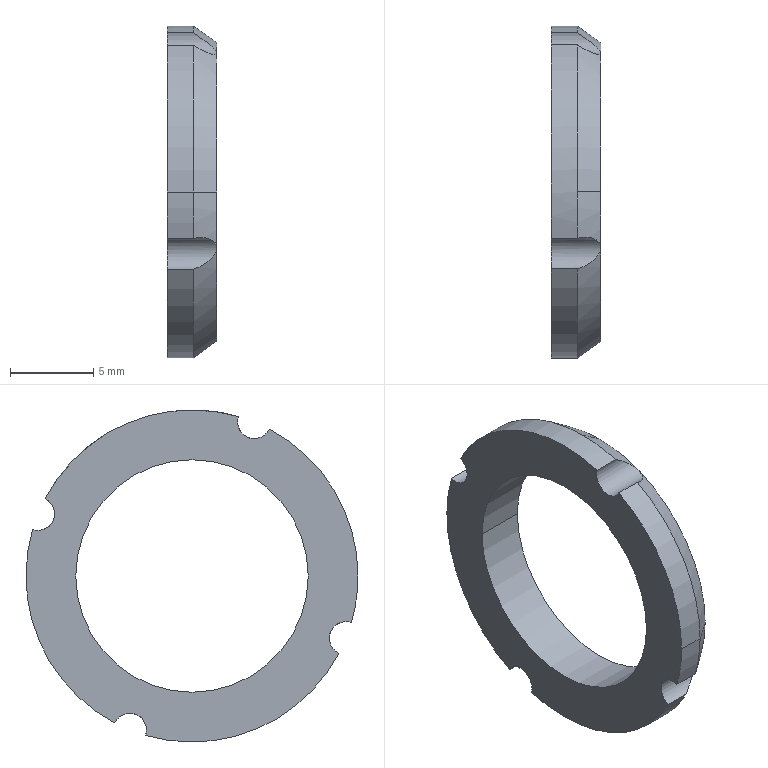Part | NX | features BREP 1 | 1 solid | 21 faces | box 3 x 20 x 20 mm | volume 423.94 mm3 | cylinder 13 | cone 6 | plane 2 | commonest cylinder face diameters 2 x6 20 x5 14 x2
STEP:
#1=CARTESIAN_POINT('',(175.452,54.835,4.588));
#2=VERTEX_POINT('',#1);
#3=CARTESIAN_POINT('',(174.139,55.415,5.496));
#4=VERTEX_POINT('',#3);
#5=CARTESIAN_POINT('',(174.139,55.415,5.496));
#6=CARTESIAN_POINT('',(174.232,55.356,5.468));
#7=CARTESIAN_POINT('',(174.396,55.257,5.406));
#8=CARTESIAN_POINT('',(174.469,55.216,5.377));
#9=CARTESIAN_POINT('',(174.702,55.091,5.263));
#10=CARTESIAN_POINT('',(174.889,55.003,5.149));
#11=CARTESIAN_POINT('',(175.183,54.878,4.941));
#12=CARTESIAN_POINT('',(175.388,54.835,4.696));
#13=CARTESIAN_POINT('',(175.452,54.835,4.588));
#14=B_SPLINE_CURVE_WITH_KNOTS('',3,(#5,#6,#7,#8,#9,#10,#11,#12,#13),.UNSPECIFIED.,.F.,.F.,(4,1,1,1,1,1,4),(0.,0.125,0.25,0.375,0.5,0.75,1.),.UNSPECIFIED.);
#15=EDGE_CURVE('',#2,#4,#14,.F.);
#16=ORIENTED_EDGE('',*,*,#15,.F.);
#17=CARTESIAN_POINT('',(172.567,54.835,4.588));
#18=VERTEX_POINT('',#17);
#19=CARTESIAN_POINT('',(175.567,54.835,4.588));
#20=DIRECTION('',(-1.,0.,0.));
#21=VECTOR('',#20,1000.);
#22=LINE('',#19,#21);
#23=EDGE_CURVE('',#2,#18,#22,.T.);
#24=ORIENTED_EDGE('',*,*,#23,.T.);
#25=CARTESIAN_POINT('',(172.567,55.415,5.496));
#26=VERTEX_POINT('',#25);
#27=CARTESIAN_POINT('',(172.567,55.835,4.588));
#28=DIRECTION('',(-1.,0.,0.));
#29=DIRECTION('',(0.,-1.,0.));
#30=AXIS2_PLACEMENT_3D('',#27,#28,#29);
#31=CIRCLE('',#30,1.);
#32=EDGE_CURVE('',#18,#26,#31,.T.);
#33=ORIENTED_EDGE('',*,*,#32,.T.);
#34=CARTESIAN_POINT('',(175.567,55.415,5.496));
#35=DIRECTION('',(-1.,0.,0.));
#36=VECTOR('',#35,1000.);
#37=LINE('',#34,#36);
#38=EDGE_CURVE('',#4,#26,#37,.T.);
#39=ORIENTED_EDGE('',*,*,#38,.F.);
#40=EDGE_LOOP('',(#16,#24,#33,#39));
#41=FACE_BOUND('',#40,.T.);
#42=CARTESIAN_POINT('',(175.567,55.835,4.588));
#43=DIRECTION('',(-1.,0.,0.));
#44=DIRECTION('',(0.,-1.,0.));
#45=AXIS2_PLACEMENT_3D('',#42,#43,#44);
#46=CYLINDRICAL_SURFACE('',#45,1.);
#47=ADVANCED_FACE('',(#41),#46,.F.);
#48=CARTESIAN_POINT('',(174.139,36.963,-1.956));
#49=VERTEX_POINT('',#48);
#50=CARTESIAN_POINT('',(174.139,36.563,0.8438));
#51=VERTEX_POINT('',#50);
#52=CARTESIAN_POINT('',(174.139,46.563,0.8438));
#53=DIRECTION('',(-1.,0.,0.));
#54=DIRECTION('',(0.,-1.,0.));
#55=AXIS2_PLACEMENT_3D('',#52,#53,#54);
#56=CIRCLE('',#55,10.);
#57=EDGE_CURVE('',#49,#51,#56,.T.);
#58=ORIENTED_EDGE('',*,*,#57,.T.);
#59=CARTESIAN_POINT('',(172.567,36.563,0.8438));
#60=VERTEX_POINT('',#59);
#61=CARTESIAN_POINT('',(175.567,36.563,0.8438));
#62=DIRECTION('',(-1.,0.,0.));
#63=VECTOR('',#62,1000.);
#64=LINE('',#61,#63);
#65=EDGE_CURVE('',#51,#60,#64,.T.);
#66=ORIENTED_EDGE('',*,*,#65,.T.);
#67=CARTESIAN_POINT('',(172.567,36.963,-1.956));
#68=VERTEX_POINT('',#67);
#69=CARTESIAN_POINT('',(172.567,46.563,0.8438));
#70=DIRECTION('',(1.,0.,0.));
#71=DIRECTION('',(0.,-1.,0.));
#72=AXIS2_PLACEMENT_3D('',#69,#70,#71);
#73=CIRCLE('',#72,10.);
#74=EDGE_CURVE('',#60,#68,#73,.T.);
#75=ORIENTED_EDGE('',*,*,#74,.T.);
#76=CARTESIAN_POINT('',(175.567,36.963,-1.956));
#77=DIRECTION('',(1.,0.,0.));
#78=VECTOR('',#77,1000.);
#79=LINE('',#76,#78);
#80=EDGE_CURVE('',#68,#49,#79,.T.);
#81=ORIENTED_EDGE('',*,*,#80,.T.);
#82=EDGE_LOOP('',(#58,#66,#75,#81));
#83=FACE_BOUND('',#82,.T.);
#84=CARTESIAN_POINT('',(175.567,46.563,0.8438));
#85=DIRECTION('',(-1.,0.,0.));
#86=DIRECTION('',(0.,-1.,0.));
#87=AXIS2_PLACEMENT_3D('',#84,#85,#86);
#88=CYLINDRICAL_SURFACE('',#87,10.);
#89=ADVANCED_FACE('',(#83),#88,.T.);
#90=CARTESIAN_POINT('',(172.567,53.563,0.8438));
#91=VERTEX_POINT('',#90);
#92=CARTESIAN_POINT('',(172.567,39.563,0.8438));
#93=VERTEX_POINT('',#92);
#94=CARTESIAN_POINT('',(172.567,46.563,0.8438));
#95=DIRECTION('',(-1.,0.,0.));
#96=DIRECTION('',(0.,1.,0.));
#97=AXIS2_PLACEMENT_3D('',#94,#95,#96);
#98=CIRCLE('',#97,7.);
#99=EDGE_CURVE('',#91,#93,#98,.T.);
#100=ORIENTED_EDGE('',*,*,#99,.T.);
#101=CARTESIAN_POINT('',(175.567,39.563,0.8438));
#102=VERTEX_POINT('',#101);
#103=CARTESIAN_POINT('',(175.567,39.563,0.8438));
#104=DIRECTION('',(1.,0.,0.));
#105=VECTOR('',#104,1000.);
#106=LINE('',#103,#105);
#107=EDGE_CURVE('',#102,#93,#106,.F.);
#108=ORIENTED_EDGE('',*,*,#107,.F.);
#109=CARTESIAN_POINT('',(175.567,53.563,0.8438));
#110=VERTEX_POINT('',#109);
#111=CARTESIAN_POINT('',(175.567,46.563,0.8438));
#112=DIRECTION('',(-1.,0.,0.));
#113=DIRECTION('',(0.,1.,0.));
#114=AXIS2_PLACEMENT_3D('',#111,#112,#113);
#115=CIRCLE('',#114,7.);
#116=EDGE_CURVE('',#110,#102,#115,.T.);
#117=ORIENTED_EDGE('',*,*,#116,.F.);
#118=CARTESIAN_POINT('',(175.567,53.563,0.8438));
#119=DIRECTION('',(1.,0.,0.));
#120=VECTOR('',#119,1000.);
#121=LINE('',#118,#120);
#122=EDGE_CURVE('',#110,#91,#121,.F.);
#123=ORIENTED_EDGE('',*,*,#122,.T.);
#124=EDGE_LOOP('',(#100,#108,#117,#123));
#125=FACE_BOUND('',#124,.T.);
#126=CARTESIAN_POINT('',(175.567,46.563,0.8438));
#127=DIRECTION('',(1.,0.,0.));
#128=DIRECTION('',(0.,1.,0.));
#129=AXIS2_PLACEMENT_3D('',#126,#127,#128);
#130=CYLINDRICAL_SURFACE('',#129,7.);
#131=ADVANCED_FACE('',(#125),#130,.F.);
#132=CARTESIAN_POINT('',(175.567,43.193,9.189));
#133=VERTEX_POINT('',#132);
#134=CARTESIAN_POINT('',(175.567,46.563,9.844));
#135=VERTEX_POINT('',#134);
#136=CARTESIAN_POINT('',(175.567,46.563,0.8438));
#137=DIRECTION('',(-1.,0.,0.));
#138=DIRECTION('',(0.,0.,1.));
#139=AXIS2_PLACEMENT_3D('',#136,#137,#138);
#140=CIRCLE('',#139,9.);
#141=EDGE_CURVE('',#133,#135,#140,.T.);
#142=ORIENTED_EDGE('',*,*,#141,.T.);
#143=CARTESIAN_POINT('',(174.139,46.563,10.844));
#144=VERTEX_POINT('',#143);
#145=CARTESIAN_POINT('',(174.139,46.563,10.844));
#146=DIRECTION('',(-0.8192,0.,0.5736));
#147=VECTOR('',#146,1000.);
#148=LINE('',#145,#147);
#149=EDGE_CURVE('',#135,#144,#148,.T.);
#150=ORIENTED_EDGE('',*,*,#149,.T.);
#151=CARTESIAN_POINT('',(174.139,43.763,10.444));
#152=VERTEX_POINT('',#151);
#153=CARTESIAN_POINT('',(174.139,46.563,0.8438));
#154=DIRECTION('',(-1.,0.,0.));
#155=DIRECTION('',(0.,-1.,0.));
#156=AXIS2_PLACEMENT_3D('',#153,#154,#155);
#157=CIRCLE('',#156,10.);
#158=EDGE_CURVE('',#152,#144,#157,.T.);
#159=ORIENTED_EDGE('',*,*,#158,.F.);
#160=CARTESIAN_POINT('',(175.567,43.193,9.189));
#161=CARTESIAN_POINT('',(175.567,43.342,9.249));
#162=CARTESIAN_POINT('',(175.424,43.576,9.441));
#163=CARTESIAN_POINT('',(175.233,43.694,9.62));
#164=CARTESIAN_POINT('',(174.983,43.783,9.833));
#165=CARTESIAN_POINT('',(174.833,43.809,9.95));
#166=CARTESIAN_POINT('',(174.544,43.821,10.165));
#167=CARTESIAN_POINT('',(174.446,43.813,10.234));
#168=CARTESIAN_POINT('',(174.249,43.788,10.371));
#169=CARTESIAN_POINT('',(174.139,43.763,10.444));
#170=B_SPLINE_CURVE_WITH_KNOTS('',3,(#160,#161,#162,#163,#164,#165,#166,#167,#168,#169),.UNSPECIFIED.,.F.,.F.,(4,1,1,1,1,1,1,4),(0.,0.25,0.375,0.5,0.625,0.75,0.875,1.),.UNSPECIFIED.);
#171=EDGE_CURVE('',#152,#133,#170,.F.);
#172=ORIENTED_EDGE('',*,*,#171,.T.);
#173=EDGE_LOOP('',(#142,#150,#159,#172));
#174=FACE_BOUND('',#173,.T.);
#175=CARTESIAN_POINT('',(174.139,46.563,0.8438));
#176=DIRECTION('',(-1.,0.,0.));
#177=DIRECTION('',(0.,0.,1.));
#178=AXIS2_PLACEMENT_3D('',#175,#176,#177);
#179=CONICAL_SURFACE('',#178,10.,0.6109);
#180=ADVANCED_FACE('',(#174),#179,.T.);
#181=CARTESIAN_POINT('',(175.567,38.218,-2.526));
#182=VERTEX_POINT('',#181);
#183=CARTESIAN_POINT('',(175.567,37.563,0.8438));
#184=VERTEX_POINT('',#183);
#185=CARTESIAN_POINT('',(175.567,46.563,0.8438));
#186=DIRECTION('',(-1.,0.,0.));
#187=DIRECTION('',(0.,-1.,0.));
#188=AXIS2_PLACEMENT_3D('',#185,#186,#187);
#189=CIRCLE('',#188,9.);
#190=EDGE_CURVE('',#182,#184,#189,.T.);
#191=ORIENTED_EDGE('',*,*,#190,.T.);
#192=CARTESIAN_POINT('',(174.139,36.563,0.8438));
#193=DIRECTION('',(-0.8192,-0.5736,0.));
#194=VECTOR('',#193,1000.);
#195=LINE('',#192,#194);
#196=EDGE_CURVE('',#184,#51,#195,.T.);
#197=ORIENTED_EDGE('',*,*,#196,.T.);
#198=ORIENTED_EDGE('',*,*,#57,.F.);
#199=CARTESIAN_POINT('',(175.567,38.218,-2.526));
#200=CARTESIAN_POINT('',(175.567,38.157,-2.377));
#201=CARTESIAN_POINT('',(175.424,37.965,-2.143));
#202=CARTESIAN_POINT('',(175.233,37.786,-2.025));
#203=CARTESIAN_POINT('',(174.983,37.574,-1.936));
#204=CARTESIAN_POINT('',(174.833,37.456,-1.91));
#205=CARTESIAN_POINT('',(174.544,37.241,-1.898));
#206=CARTESIAN_POINT('',(174.446,37.173,-1.906));
#207=CARTESIAN_POINT('',(174.249,37.035,-1.931));
#208=CARTESIAN_POINT('',(174.139,36.963,-1.956));
#209=B_SPLINE_CURVE_WITH_KNOTS('',3,(#199,#200,#201,#202,#203,#204,#205,#206,#207,#208),.UNSPECIFIED.,.F.,.F.,(4,1,1,1,1,1,1,4),(0.,0.25,0.375,0.5,0.625,0.75,0.875,1.),.UNSPECIFIED.);
#210=EDGE_CURVE('',#49,#182,#209,.F.);
#211=ORIENTED_EDGE('',*,*,#210,.T.);
#212=EDGE_LOOP('',(#191,#197,#198,#211));
#213=FACE_BOUND('',#212,.T.);
#214=CARTESIAN_POINT('',(174.139,46.563,0.8438));
#215=DIRECTION('',(-1.,0.,0.));
#216=DIRECTION('',(0.,-1.,0.));
#217=AXIS2_PLACEMENT_3D('',#214,#215,#216);
#218=CONICAL_SURFACE('',#217,10.,0.6109);
#219=ADVANCED_FACE('',(#213),#218,.T.);
#220=CARTESIAN_POINT('',(174.61,49.307,-8.429));
#221=VERTEX_POINT('',#220);
#222=CARTESIAN_POINT('',(175.567,49.933,-7.501));
#223=VERTEX_POINT('',#222);
#224=CARTESIAN_POINT('',(175.567,49.933,-7.501));
#225=CARTESIAN_POINT('',(175.567,49.705,-7.594));
#226=CARTESIAN_POINT('',(175.22,49.356,-7.971));
#227=CARTESIAN_POINT('',(174.848,49.307,-8.255));
#228=CARTESIAN_POINT('',(174.61,49.307,-8.429));
#229=B_SPLINE_CURVE_WITH_KNOTS('',3,(#224,#225,#226,#227,#228),.UNSPECIFIED.,.F.,.F.,(4,1,4),(0.,0.5,1.),.UNSPECIFIED.);
#230=EDGE_CURVE('',#221,#223,#229,.F.);
#231=ORIENTED_EDGE('',*,*,#230,.F.);
#232=CARTESIAN_POINT('',(172.567,49.307,-8.429));
#233=VERTEX_POINT('',#232);
#234=CARTESIAN_POINT('',(175.567,49.307,-8.429));
#235=DIRECTION('',(-1.,0.,0.));
#236=VECTOR('',#235,1000.);
#237=LINE('',#234,#236);
#238=EDGE_CURVE('',#221,#233,#237,.T.);
#239=ORIENTED_EDGE('',*,*,#238,.T.);
#240=CARTESIAN_POINT('',(172.567,51.215,-8.008));
#241=VERTEX_POINT('',#240);
#242=CARTESIAN_POINT('',(172.567,50.307,-8.429));
#243=DIRECTION('',(1.,0.,0.));
#244=DIRECTION('',(0.,-1.,0.));
#245=AXIS2_PLACEMENT_3D('',#242,#243,#244);
#246=CIRCLE('',#245,1.);
#247=EDGE_CURVE('',#241,#233,#246,.T.);
#248=ORIENTED_EDGE('',*,*,#247,.F.);
#249=CARTESIAN_POINT('',(174.139,51.215,-8.008));
#250=VERTEX_POINT('',#249);
#251=CARTESIAN_POINT('',(175.567,51.215,-8.008));
#252=DIRECTION('',(-1.,0.,0.));
#253=VECTOR('',#252,1000.);
#254=LINE('',#251,#253);
#255=EDGE_CURVE('',#250,#241,#254,.T.);
#256=ORIENTED_EDGE('',*,*,#255,.F.);
#257=CARTESIAN_POINT('',(174.139,51.215,-8.008));
#258=CARTESIAN_POINT('',(174.249,51.182,-7.938));
#259=CARTESIAN_POINT('',(174.446,51.105,-7.822));
#260=CARTESIAN_POINT('',(174.546,51.063,-7.767));
#261=CARTESIAN_POINT('',(174.834,50.905,-7.62));
#262=CARTESIAN_POINT('',(174.986,50.803,-7.554));
#263=CARTESIAN_POINT('',(175.234,50.592,-7.464));
#264=CARTESIAN_POINT('',(175.424,50.384,-7.417));
#265=CARTESIAN_POINT('',(175.567,50.082,-7.441));
#266=CARTESIAN_POINT('',(175.567,49.933,-7.501));
#267=B_SPLINE_CURVE_WITH_KNOTS('',3,(#257,#258,#259,#260,#261,#262,#263,#264,#265,#266),.UNSPECIFIED.,.F.,.F.,(4,1,1,1,1,1,1,4),(0.,0.125,0.25,0.375,0.5,0.625,0.75,1.),.UNSPECIFIED.);
#268=EDGE_CURVE('',#223,#250,#267,.F.);
#269=ORIENTED_EDGE('',*,*,#268,.F.);
#270=EDGE_LOOP('',(#231,#239,#248,#256,#269));
#271=FACE_BOUND('',#270,.T.);
#272=CARTESIAN_POINT('',(175.567,50.307,-8.429));
#273=DIRECTION('',(-1.,0.,0.));
#274=DIRECTION('',(0.,-1.,0.));
#275=AXIS2_PLACEMENT_3D('',#272,#273,#274);
#276=CYLINDRICAL_SURFACE('',#275,1.);
#277=ADVANCED_FACE('',(#271),#276,.F.);
#278=CARTESIAN_POINT('',(172.567,56.163,3.644));
#279=VERTEX_POINT('',#278);
#280=CARTESIAN_POINT('',(172.567,55.835,4.588));
#281=DIRECTION('',(-1.,0.,0.));
#282=DIRECTION('',(0.,-1.,0.));
#283=AXIS2_PLACEMENT_3D('',#280,#281,#282);
#284=CIRCLE('',#283,1.);
#285=EDGE_CURVE('',#279,#18,#284,.T.);
#286=ORIENTED_EDGE('',*,*,#285,.F.);
#287=CARTESIAN_POINT('',(172.567,46.563,0.8438));
#288=DIRECTION('',(1.,0.,0.));
#289=DIRECTION('',(0.,-1.,0.));
#290=AXIS2_PLACEMENT_3D('',#287,#288,#289);
#291=CIRCLE('',#290,10.);
#292=EDGE_CURVE('',#241,#279,#291,.T.);
#293=ORIENTED_EDGE('',*,*,#292,.F.);
#294=ORIENTED_EDGE('',*,*,#247,.T.);
#295=CARTESIAN_POINT('',(172.567,49.363,-8.756));
#296=VERTEX_POINT('',#295);
#297=CARTESIAN_POINT('',(172.567,50.307,-8.429));
#298=DIRECTION('',(1.,0.,0.));
#299=DIRECTION('',(0.,-1.,0.));
#300=AXIS2_PLACEMENT_3D('',#297,#298,#299);
#301=CIRCLE('',#300,1.);
#302=EDGE_CURVE('',#233,#296,#301,.T.);
#303=ORIENTED_EDGE('',*,*,#302,.T.);
#304=CARTESIAN_POINT('',(172.567,37.711,-3.808));
#305=VERTEX_POINT('',#304);
#306=CARTESIAN_POINT('',(172.567,46.563,0.8438));
#307=DIRECTION('',(1.,0.,0.));
#308=DIRECTION('',(0.,-1.,0.));
#309=AXIS2_PLACEMENT_3D('',#306,#307,#308);
#310=CIRCLE('',#309,10.);
#311=EDGE_CURVE('',#305,#296,#310,.T.);
#312=ORIENTED_EDGE('',*,*,#311,.F.);
#313=CARTESIAN_POINT('',(172.567,37.29,-2.901));
#314=DIRECTION('',(-1.,0.,0.));
#315=DIRECTION('',(0.,-1.,0.));
#316=AXIS2_PLACEMENT_3D('',#313,#314,#315);
#317=CIRCLE('',#316,1.);
#318=EDGE_CURVE('',#68,#305,#317,.T.);
#319=ORIENTED_EDGE('',*,*,#318,.F.);
#320=ORIENTED_EDGE('',*,*,#74,.F.);
#321=CARTESIAN_POINT('',(172.567,41.911,9.696));
#322=VERTEX_POINT('',#321);
#323=CARTESIAN_POINT('',(172.567,46.563,0.8438));
#324=DIRECTION('',(1.,0.,0.));
#325=DIRECTION('',(0.,-1.,0.));
#326=AXIS2_PLACEMENT_3D('',#323,#324,#325);
#327=CIRCLE('',#326,10.);
#328=EDGE_CURVE('',#322,#60,#327,.T.);
#329=ORIENTED_EDGE('',*,*,#328,.F.);
#330=CARTESIAN_POINT('',(172.567,43.763,10.444));
#331=VERTEX_POINT('',#330);
#332=CARTESIAN_POINT('',(172.567,42.818,10.116));
#333=DIRECTION('',(-1.,0.,0.));
#334=DIRECTION('',(0.,-1.,0.));
#335=AXIS2_PLACEMENT_3D('',#332,#333,#334);
#336=CIRCLE('',#335,1.);
#337=EDGE_CURVE('',#331,#322,#336,.T.);
#338=ORIENTED_EDGE('',*,*,#337,.F.);
#339=CARTESIAN_POINT('',(172.567,46.563,0.8438));
#340=DIRECTION('',(1.,0.,0.));
#341=DIRECTION('',(0.,-1.,0.));
#342=AXIS2_PLACEMENT_3D('',#339,#340,#341);
#343=CIRCLE('',#342,10.);
#344=EDGE_CURVE('',#26,#331,#343,.T.);
#345=ORIENTED_EDGE('',*,*,#344,.F.);
#346=ORIENTED_EDGE('',*,*,#32,.F.);
#347=EDGE_LOOP('',(#286,#293,#294,#303,#312,#319,#320,#329,#338,#345,#346));
#348=FACE_BOUND('',#347,.T.);
#349=ORIENTED_EDGE('',*,*,#99,.F.);
#350=CARTESIAN_POINT('',(172.567,46.563,0.8438));
#351=DIRECTION('',(-1.,0.,0.));
#352=DIRECTION('',(0.,1.,0.));
#353=AXIS2_PLACEMENT_3D('',#350,#351,#352);
#354=CIRCLE('',#353,7.);
#355=EDGE_CURVE('',#93,#91,#354,.T.);
#356=ORIENTED_EDGE('',*,*,#355,.F.);
#357=EDGE_LOOP('',(#349,#356));
#358=FACE_BOUND('',#357,.T.);
#359=CARTESIAN_POINT('',(172.567,46.563,0.8438));
#360=DIRECTION('',(1.,0.,0.));
#361=DIRECTION('',(0.,-1.,0.));
#362=AXIS2_PLACEMENT_3D('',#359,#360,#361);
#363=PLANE('',#362);
#364=ADVANCED_FACE('',(#348,#358),#363,.F.);
#365=ORIENTED_EDGE('',*,*,#344,.T.);
#366=CARTESIAN_POINT('',(175.567,43.763,10.444));
#367=DIRECTION('',(1.,0.,0.));
#368=VECTOR('',#367,1000.);
#369=LINE('',#366,#368);
#370=EDGE_CURVE('',#331,#152,#369,.T.);
#371=ORIENTED_EDGE('',*,*,#370,.T.);
#372=ORIENTED_EDGE('',*,*,#158,.T.);
#373=CARTESIAN_POINT('',(174.139,46.563,0.8438));
#374=DIRECTION('',(-1.,0.,0.));
#375=DIRECTION('',(0.,-1.,0.));
#376=AXIS2_PLACEMENT_3D('',#373,#374,#375);
#377=CIRCLE('',#376,10.);
#378=EDGE_CURVE('',#144,#4,#377,.T.);
#379=ORIENTED_EDGE('',*,*,#378,.T.);
#380=ORIENTED_EDGE('',*,*,#38,.T.);
#381=EDGE_LOOP('',(#365,#371,#372,#379,#380));
#382=FACE_BOUND('',#381,.T.);
#383=CARTESIAN_POINT('',(175.567,46.563,0.8438));
#384=DIRECTION('',(-1.,0.,0.));
#385=DIRECTION('',(0.,-1.,0.));
#386=AXIS2_PLACEMENT_3D('',#383,#384,#385);
#387=CYLINDRICAL_SURFACE('',#386,10.);
#388=ADVANCED_FACE('',(#382),#387,.T.);
#389=ORIENTED_EDGE('',*,*,#23,.F.);
#390=CARTESIAN_POINT('',(175.567,54.908,4.214));
#391=VERTEX_POINT('',#390);
#392=CARTESIAN_POINT('',(175.452,54.835,4.588));
#393=CARTESIAN_POINT('',(175.529,54.835,4.458));
#394=CARTESIAN_POINT('',(175.567,54.861,4.331));
#395=CARTESIAN_POINT('',(175.567,54.908,4.214));
#396=B_SPLINE_CURVE_WITH_KNOTS('',3,(#392,#393,#394,#395),.UNSPECIFIED.,.F.,.F.,(4,4),(0.,1.),.UNSPECIFIED.);
#397=EDGE_CURVE('',#391,#2,#396,.F.);
#398=ORIENTED_EDGE('',*,*,#397,.F.);
#399=CARTESIAN_POINT('',(174.139,56.163,3.644));
#400=VERTEX_POINT('',#399);
#401=CARTESIAN_POINT('',(175.567,54.908,4.214));
#402=CARTESIAN_POINT('',(175.567,54.968,4.065));
#403=CARTESIAN_POINT('',(175.424,55.16,3.83));
#404=CARTESIAN_POINT('',(175.233,55.339,3.713));
#405=CARTESIAN_POINT('',(174.983,55.552,3.624));
#406=CARTESIAN_POINT('',(174.833,55.669,3.597));
#407=CARTESIAN_POINT('',(174.544,55.884,3.585));
#408=CARTESIAN_POINT('',(174.446,55.953,3.593));
#409=CARTESIAN_POINT('',(174.249,56.09,3.618));
#410=CARTESIAN_POINT('',(174.139,56.163,3.644));
#411=B_SPLINE_CURVE_WITH_KNOTS('',3,(#401,#402,#403,#404,#405,#406,#407,#408,#409,#410),.UNSPECIFIED.,.F.,.F.,(4,1,1,1,1,1,1,4),(0.,0.25,0.375,0.5,0.625,0.75,0.875,1.),.UNSPECIFIED.);
#412=EDGE_CURVE('',#400,#391,#411,.F.);
#413=ORIENTED_EDGE('',*,*,#412,.F.);
#414=CARTESIAN_POINT('',(175.567,56.163,3.644));
#415=DIRECTION('',(1.,0.,0.));
#416=VECTOR('',#415,1000.);
#417=LINE('',#414,#416);
#418=EDGE_CURVE('',#279,#400,#417,.T.);
#419=ORIENTED_EDGE('',*,*,#418,.F.);
#420=ORIENTED_EDGE('',*,*,#285,.T.);
#421=EDGE_LOOP('',(#389,#398,#413,#419,#420));
#422=FACE_BOUND('',#421,.T.);
#423=CARTESIAN_POINT('',(175.567,55.835,4.588));
#424=DIRECTION('',(-1.,0.,0.));
#425=DIRECTION('',(0.,-1.,0.));
#426=AXIS2_PLACEMENT_3D('',#423,#424,#425);
#427=CYLINDRICAL_SURFACE('',#426,1.);
#428=ADVANCED_FACE('',(#422),#427,.F.);
#429=CARTESIAN_POINT('',(174.139,46.563,0.8438));
#430=DIRECTION('',(-1.,0.,0.));
#431=DIRECTION('',(0.,-1.,0.));
#432=AXIS2_PLACEMENT_3D('',#429,#430,#431);
#433=CIRCLE('',#432,10.);
#434=EDGE_CURVE('',#400,#250,#433,.T.);
#435=ORIENTED_EDGE('',*,*,#434,.T.);
#436=ORIENTED_EDGE('',*,*,#255,.T.);
#437=ORIENTED_EDGE('',*,*,#292,.T.);
#438=ORIENTED_EDGE('',*,*,#418,.T.);
#439=EDGE_LOOP('',(#435,#436,#437,#438));
#440=FACE_BOUND('',#439,.T.);
#441=CARTESIAN_POINT('',(175.567,46.563,0.8438));
#442=DIRECTION('',(-1.,0.,0.));
#443=DIRECTION('',(0.,-1.,0.));
#444=AXIS2_PLACEMENT_3D('',#441,#442,#443);
#445=CYLINDRICAL_SURFACE('',#444,10.);
#446=ADVANCED_FACE('',(#440),#445,.T.);
#447=ORIENTED_EDGE('',*,*,#311,.T.);
#448=CARTESIAN_POINT('',(174.139,49.363,-8.756));
#449=VERTEX_POINT('',#448);
#450=CARTESIAN_POINT('',(175.567,49.363,-8.756));
#451=DIRECTION('',(1.,0.,0.));
#452=VECTOR('',#451,1000.);
#453=LINE('',#450,#452);
#454=EDGE_CURVE('',#296,#449,#453,.T.);
#455=ORIENTED_EDGE('',*,*,#454,.T.);
#456=CARTESIAN_POINT('',(174.139,37.711,-3.808));
#457=VERTEX_POINT('',#456);
#458=CARTESIAN_POINT('',(174.139,46.563,0.8438));
#459=DIRECTION('',(-1.,0.,0.));
#460=DIRECTION('',(0.,-1.,0.));
#461=AXIS2_PLACEMENT_3D('',#458,#459,#460);
#462=CIRCLE('',#461,10.);
#463=EDGE_CURVE('',#449,#457,#462,.T.);
#464=ORIENTED_EDGE('',*,*,#463,.T.);
#465=CARTESIAN_POINT('',(175.567,37.711,-3.808));
#466=DIRECTION('',(-1.,0.,0.));
#467=VECTOR('',#466,1000.);
#468=LINE('',#465,#467);
#469=EDGE_CURVE('',#457,#305,#468,.T.);
#470=ORIENTED_EDGE('',*,*,#469,.T.);
#471=EDGE_LOOP('',(#447,#455,#464,#470));
#472=FACE_BOUND('',#471,.T.);
#473=CARTESIAN_POINT('',(175.567,46.563,0.8438));
#474=DIRECTION('',(-1.,0.,0.));
#475=DIRECTION('',(0.,-1.,0.));
#476=AXIS2_PLACEMENT_3D('',#473,#474,#475);
#477=CYLINDRICAL_SURFACE('',#476,10.);
#478=ADVANCED_FACE('',(#472),#477,.T.);
#479=ORIENTED_EDGE('',*,*,#469,.F.);
#480=CARTESIAN_POINT('',(174.139,37.711,-3.808));
#481=CARTESIAN_POINT('',(174.249,37.781,-3.776));
#482=CARTESIAN_POINT('',(174.446,37.897,-3.698));
#483=CARTESIAN_POINT('',(174.546,37.952,-3.656));
#484=CARTESIAN_POINT('',(174.834,38.099,-3.498));
#485=CARTESIAN_POINT('',(174.986,38.165,-3.396));
#486=CARTESIAN_POINT('',(175.234,38.255,-3.186));
#487=CARTESIAN_POINT('',(175.424,38.302,-2.978));
#488=CARTESIAN_POINT('',(175.567,38.278,-2.676));
#489=CARTESIAN_POINT('',(175.567,38.218,-2.526));
#490=B_SPLINE_CURVE_WITH_KNOTS('',3,(#480,#481,#482,#483,#484,#485,#486,#487,#488,#489),.UNSPECIFIED.,.F.,.F.,(4,1,1,1,1,1,1,4),(0.,0.125,0.25,0.375,0.5,0.625,0.75,1.),.UNSPECIFIED.);
#491=EDGE_CURVE('',#182,#457,#490,.F.);
#492=ORIENTED_EDGE('',*,*,#491,.F.);
#493=ORIENTED_EDGE('',*,*,#210,.F.);
#494=ORIENTED_EDGE('',*,*,#80,.F.);
#495=ORIENTED_EDGE('',*,*,#318,.T.);
#496=EDGE_LOOP('',(#479,#492,#493,#494,#495));
#497=FACE_BOUND('',#496,.T.);
#498=CARTESIAN_POINT('',(175.567,37.29,-2.901));
#499=DIRECTION('',(-1.,0.,0.));
#500=DIRECTION('',(0.,-1.,0.));
#501=AXIS2_PLACEMENT_3D('',#498,#499,#500);
#502=CYLINDRICAL_SURFACE('',#501,1.);
#503=ADVANCED_FACE('',(#497),#502,.F.);
#504=ORIENTED_EDGE('',*,*,#65,.F.);
#505=CARTESIAN_POINT('',(174.139,41.911,9.696));
#506=VERTEX_POINT('',#505);
#507=CARTESIAN_POINT('',(174.139,46.563,0.8438));
#508=DIRECTION('',(-1.,0.,0.));
#509=DIRECTION('',(0.,-1.,0.));
#510=AXIS2_PLACEMENT_3D('',#507,#508,#509);
#511=CIRCLE('',#510,10.);
#512=EDGE_CURVE('',#51,#506,#511,.T.);
#513=ORIENTED_EDGE('',*,*,#512,.T.);
#514=CARTESIAN_POINT('',(175.567,41.911,9.696));
#515=DIRECTION('',(-1.,0.,0.));
#516=VECTOR('',#515,1000.);
#517=LINE('',#514,#516);
#518=EDGE_CURVE('',#506,#322,#517,.T.);
#519=ORIENTED_EDGE('',*,*,#518,.T.);
#520=ORIENTED_EDGE('',*,*,#328,.T.);
#521=EDGE_LOOP('',(#504,#513,#519,#520));
#522=FACE_BOUND('',#521,.T.);
#523=CARTESIAN_POINT('',(175.567,46.563,0.8438));
#524=DIRECTION('',(-1.,0.,0.));
#525=DIRECTION('',(0.,-1.,0.));
#526=AXIS2_PLACEMENT_3D('',#523,#524,#525);
#527=CYLINDRICAL_SURFACE('',#526,10.);
#528=ADVANCED_FACE('',(#522),#527,.T.);
#529=ORIENTED_EDGE('',*,*,#518,.F.);
#530=CARTESIAN_POINT('',(174.139,41.911,9.696));
#531=CARTESIAN_POINT('',(174.249,41.943,9.626));
#532=CARTESIAN_POINT('',(174.446,42.021,9.51));
#533=CARTESIAN_POINT('',(174.546,42.063,9.454));
#534=CARTESIAN_POINT('',(174.834,42.221,9.308));
#535=CARTESIAN_POINT('',(174.986,42.323,9.241));
#536=CARTESIAN_POINT('',(175.234,42.533,9.151));
#537=CARTESIAN_POINT('',(175.424,42.741,9.104));
#538=CARTESIAN_POINT('',(175.567,43.043,9.129));
#539=CARTESIAN_POINT('',(175.567,43.193,9.189));
#540=B_SPLINE_CURVE_WITH_KNOTS('',3,(#530,#531,#532,#533,#534,#535,#536,#537,#538,#539),.UNSPECIFIED.,.F.,.F.,(4,1,1,1,1,1,1,4),(0.,0.125,0.25,0.375,0.5,0.625,0.75,1.),.UNSPECIFIED.);
#541=EDGE_CURVE('',#133,#506,#540,.F.);
#542=ORIENTED_EDGE('',*,*,#541,.F.);
#543=ORIENTED_EDGE('',*,*,#171,.F.);
#544=ORIENTED_EDGE('',*,*,#370,.F.);
#545=ORIENTED_EDGE('',*,*,#337,.T.);
#546=EDGE_LOOP('',(#529,#542,#543,#544,#545));
#547=FACE_BOUND('',#546,.T.);
#548=CARTESIAN_POINT('',(175.567,42.818,10.116));
#549=DIRECTION('',(-1.,0.,0.));
#550=DIRECTION('',(0.,-1.,0.));
#551=AXIS2_PLACEMENT_3D('',#548,#549,#550);
#552=CYLINDRICAL_SURFACE('',#551,1.);
#553=ADVANCED_FACE('',(#547),#552,.F.);
#554=ORIENTED_EDGE('',*,*,#107,.T.);
#555=ORIENTED_EDGE('',*,*,#355,.T.);
#556=ORIENTED_EDGE('',*,*,#122,.F.);
#557=CARTESIAN_POINT('',(175.567,46.563,0.8438));
#558=DIRECTION('',(-1.,0.,0.));
#559=DIRECTION('',(0.,1.,0.));
#560=AXIS2_PLACEMENT_3D('',#557,#558,#559);
#561=CIRCLE('',#560,7.);
#562=EDGE_CURVE('',#102,#110,#561,.T.);
#563=ORIENTED_EDGE('',*,*,#562,.F.);
#564=EDGE_LOOP('',(#554,#555,#556,#563));
#565=FACE_BOUND('',#564,.T.);
#566=CARTESIAN_POINT('',(175.567,46.563,0.8438));
#567=DIRECTION('',(1.,0.,0.));
#568=DIRECTION('',(0.,1.,0.));
#569=AXIS2_PLACEMENT_3D('',#566,#567,#568);
#570=CYLINDRICAL_SURFACE('',#569,7.);
#571=ADVANCED_FACE('',(#565),#570,.F.);
#572=ORIENTED_EDGE('',*,*,#149,.F.);
#573=CARTESIAN_POINT('',(175.567,46.563,0.8438));
#574=DIRECTION('',(-1.,0.,0.));
#575=DIRECTION('',(0.,0.,1.));
#576=AXIS2_PLACEMENT_3D('',#573,#574,#575);
#577=CIRCLE('',#576,9.);
#578=EDGE_CURVE('',#135,#391,#577,.T.);
#579=ORIENTED_EDGE('',*,*,#578,.T.);
#580=ORIENTED_EDGE('',*,*,#397,.T.);
#581=ORIENTED_EDGE('',*,*,#15,.T.);
#582=ORIENTED_EDGE('',*,*,#378,.F.);
#583=EDGE_LOOP('',(#572,#579,#580,#581,#582));
#584=FACE_BOUND('',#583,.T.);
#585=CARTESIAN_POINT('',(174.139,46.563,0.8438));
#586=DIRECTION('',(-1.,0.,0.));
#587=DIRECTION('',(0.,0.,1.));
#588=AXIS2_PLACEMENT_3D('',#585,#586,#587);
#589=CONICAL_SURFACE('',#588,10.,0.6109);
#590=ADVANCED_FACE('',(#584),#589,.T.);
#591=ORIENTED_EDGE('',*,*,#268,.T.);
#592=ORIENTED_EDGE('',*,*,#434,.F.);
#593=ORIENTED_EDGE('',*,*,#412,.T.);
#594=CARTESIAN_POINT('',(175.567,46.563,0.8438));
#595=DIRECTION('',(-1.,0.,0.));
#596=DIRECTION('',(0.,0.,1.));
#597=AXIS2_PLACEMENT_3D('',#594,#595,#596);
#598=CIRCLE('',#597,9.);
#599=EDGE_CURVE('',#391,#223,#598,.T.);
#600=ORIENTED_EDGE('',*,*,#599,.T.);
#601=EDGE_LOOP('',(#591,#592,#593,#600));
#602=FACE_BOUND('',#601,.T.);
#603=CARTESIAN_POINT('',(174.139,46.563,0.8438));
#604=DIRECTION('',(-1.,0.,0.));
#605=DIRECTION('',(0.,0.,1.));
#606=AXIS2_PLACEMENT_3D('',#603,#604,#605);
#607=CONICAL_SURFACE('',#606,10.,0.6109);
#608=ADVANCED_FACE('',(#602),#607,.T.);
#609=CARTESIAN_POINT('',(174.61,49.307,-8.429));
#610=CARTESIAN_POINT('',(174.47,49.307,-8.531));
#611=CARTESIAN_POINT('',(174.397,49.303,-8.585));
#612=CARTESIAN_POINT('',(174.139,49.363,-8.756));
#613=B_SPLINE_CURVE_WITH_KNOTS('',3,(#609,#610,#611,#612),.UNSPECIFIED.,.F.,.F.,(4,4),(0.,1.),.UNSPECIFIED.);
#614=EDGE_CURVE('',#449,#221,#613,.F.);
#615=ORIENTED_EDGE('',*,*,#614,.T.);
#616=ORIENTED_EDGE('',*,*,#230,.T.);
#617=CARTESIAN_POINT('',(175.567,46.563,0.8438));
#618=DIRECTION('',(-1.,0.,0.));
#619=DIRECTION('',(0.,-1.,0.));
#620=AXIS2_PLACEMENT_3D('',#617,#618,#619);
#621=CIRCLE('',#620,9.);
#622=EDGE_CURVE('',#223,#182,#621,.T.);
#623=ORIENTED_EDGE('',*,*,#622,.T.);
#624=ORIENTED_EDGE('',*,*,#491,.T.);
#625=ORIENTED_EDGE('',*,*,#463,.F.);
#626=EDGE_LOOP('',(#615,#616,#623,#624,#625));
#627=FACE_BOUND('',#626,.T.);
#628=CARTESIAN_POINT('',(174.139,46.563,0.8438));
#629=DIRECTION('',(-1.,0.,0.));
#630=DIRECTION('',(0.,-1.,0.));
#631=AXIS2_PLACEMENT_3D('',#628,#629,#630);
#632=CONICAL_SURFACE('',#631,10.,0.6109);
#633=ADVANCED_FACE('',(#627),#632,.T.);
#634=ORIENTED_EDGE('',*,*,#196,.F.);
#635=CARTESIAN_POINT('',(175.567,46.563,0.8438));
#636=DIRECTION('',(-1.,0.,0.));
#637=DIRECTION('',(0.,-1.,0.));
#638=AXIS2_PLACEMENT_3D('',#635,#636,#637);
#639=CIRCLE('',#638,9.);
#640=EDGE_CURVE('',#184,#133,#639,.T.);
#641=ORIENTED_EDGE('',*,*,#640,.T.);
#642=ORIENTED_EDGE('',*,*,#541,.T.);
#643=ORIENTED_EDGE('',*,*,#512,.F.);
#644=EDGE_LOOP('',(#634,#641,#642,#643));
#645=FACE_BOUND('',#644,.T.);
#646=CARTESIAN_POINT('',(174.139,46.563,0.8438));
#647=DIRECTION('',(-1.,0.,0.));
#648=DIRECTION('',(0.,-1.,0.));
#649=AXIS2_PLACEMENT_3D('',#646,#647,#648);
#650=CONICAL_SURFACE('',#649,10.,0.6109);
#651=ADVANCED_FACE('',(#645),#650,.T.);
#652=ORIENTED_EDGE('',*,*,#190,.F.);
#653=ORIENTED_EDGE('',*,*,#622,.F.);
#654=ORIENTED_EDGE('',*,*,#599,.F.);
#655=ORIENTED_EDGE('',*,*,#578,.F.);
#656=ORIENTED_EDGE('',*,*,#141,.F.);
#657=ORIENTED_EDGE('',*,*,#640,.F.);
#658=EDGE_LOOP('',(#652,#653,#654,#655,#656,#657));
#659=FACE_BOUND('',#658,.T.);
#660=ORIENTED_EDGE('',*,*,#116,.T.);
#661=ORIENTED_EDGE('',*,*,#562,.T.);
#662=EDGE_LOOP('',(#660,#661));
#663=FACE_BOUND('',#662,.T.);
#664=CARTESIAN_POINT('',(175.567,46.563,0.8438));
#665=DIRECTION('',(1.,0.,0.));
#666=DIRECTION('',(0.,-1.,0.));
#667=AXIS2_PLACEMENT_3D('',#664,#665,#666);
#668=PLANE('',#667);
#669=ADVANCED_FACE('',(#659,#663),#668,.T.);
#670=ORIENTED_EDGE('',*,*,#238,.F.);
#671=ORIENTED_EDGE('',*,*,#614,.F.);
#672=ORIENTED_EDGE('',*,*,#454,.F.);
#673=ORIENTED_EDGE('',*,*,#302,.F.);
#674=EDGE_LOOP('',(#670,#671,#672,#673));
#675=FACE_BOUND('',#674,.T.);
#676=CARTESIAN_POINT('',(175.567,50.307,-8.429));
#677=DIRECTION('',(-1.,0.,0.));
#678=DIRECTION('',(0.,-1.,0.));
#679=AXIS2_PLACEMENT_3D('',#676,#677,#678);
#680=CYLINDRICAL_SURFACE('',#679,1.);
#681=ADVANCED_FACE('',(#675),#680,.F.);
#682=CLOSED_SHELL('',(#47,#89,#131,#180,#219,#277,#364,#388,#428,#446,#478,#503,#528,#553,#571,#590,#608,#633,#651,#669,#681));
#683=MANIFOLD_SOLID_BREP('',#682);
#684=(LENGTH_UNIT()NAMED_UNIT(*)SI_UNIT(.MILLI.,.METRE.));
#685=UNCERTAINTY_MEASURE_WITH_UNIT(LENGTH_MEASURE(0.0508),#684,'','');
#686=(NAMED_UNIT(*)PLANE_ANGLE_UNIT()SI_UNIT($,.RADIAN.));
#687=(NAMED_UNIT(*)SI_UNIT($,.STERADIAN.)SOLID_ANGLE_UNIT());
#688=(GEOMETRIC_REPRESENTATION_CONTEXT(3)GLOBAL_UNCERTAINTY_ASSIGNED_CONTEXT((#685))GLOBAL_UNIT_ASSIGNED_CONTEXT((#684,#686,#687))REPRESENTATION_CONTEXT('',''));
#689=ADVANCED_BREP_SHAPE_REPRESENTATION('',(#683),#688);